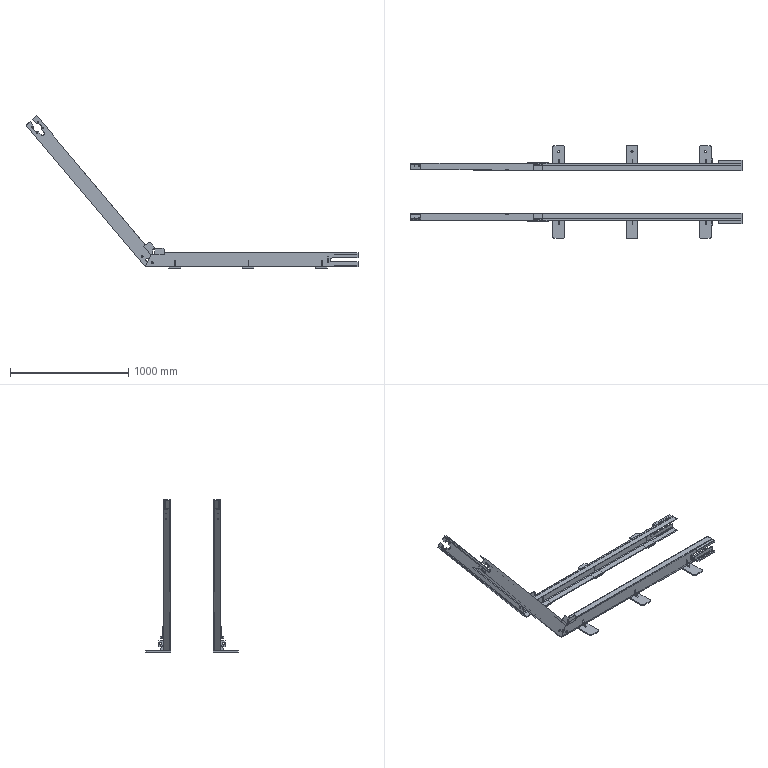Part | STEP file | mniejszy podajnik1V11_Default<Obrobiona> | 24 solids | 308 faces | box 2807 x 780 x 1287 mm | volume 9743020 mm3 | plane 204 | cylinder 104 | commonest cylinder face diameters 20 x20 16 x18 12 x16 17 x12 8.5 x8 25 x8